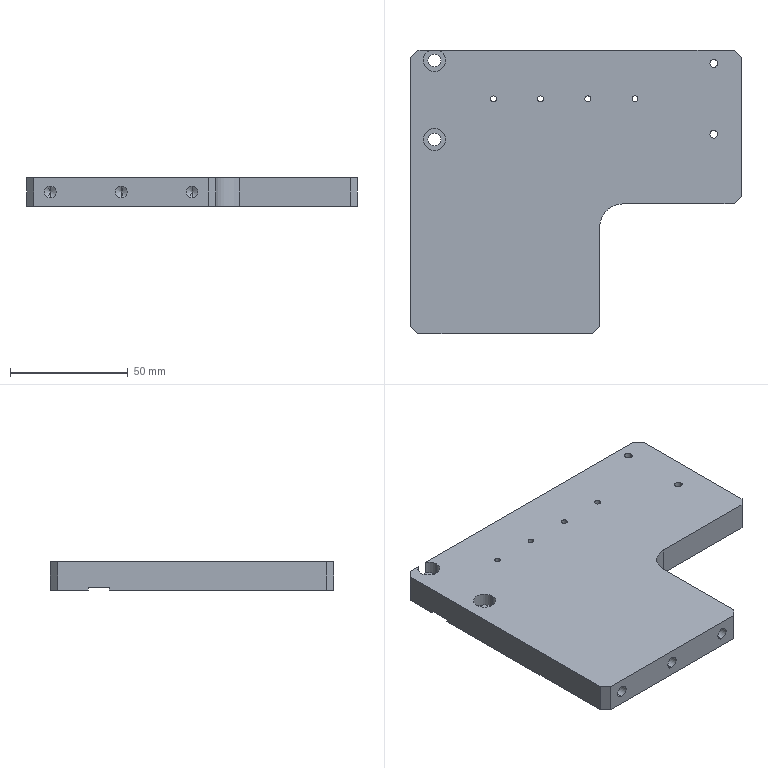Part | STEP file | Shift support plate_Default | 1 solid | 61 faces | box 140 x 120 x 12 mm | volume 158109 mm3 | cylinder 32 | plane 19 | cone 10 | commonest cylinder face diameters 2.5 x12 5 x6 9.5 x5 3.3 x4 5.5 x4 20 x1